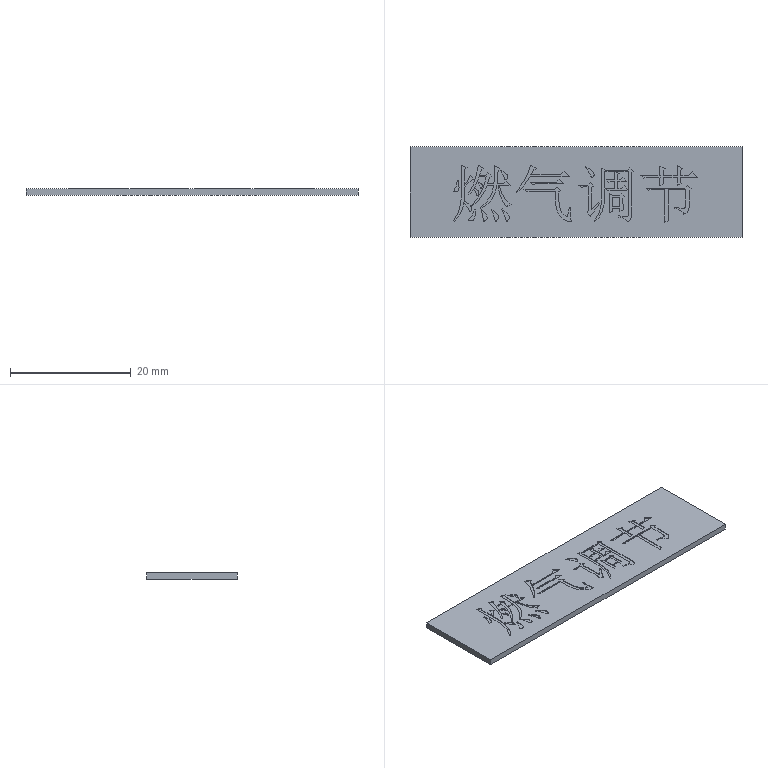Part | STEP file | HXGR200008-06-02-05 | 1 solid | 254 faces | box 55 x 15 x 1 mm | volume 817.796 mm3 | plane 162 | spline 92